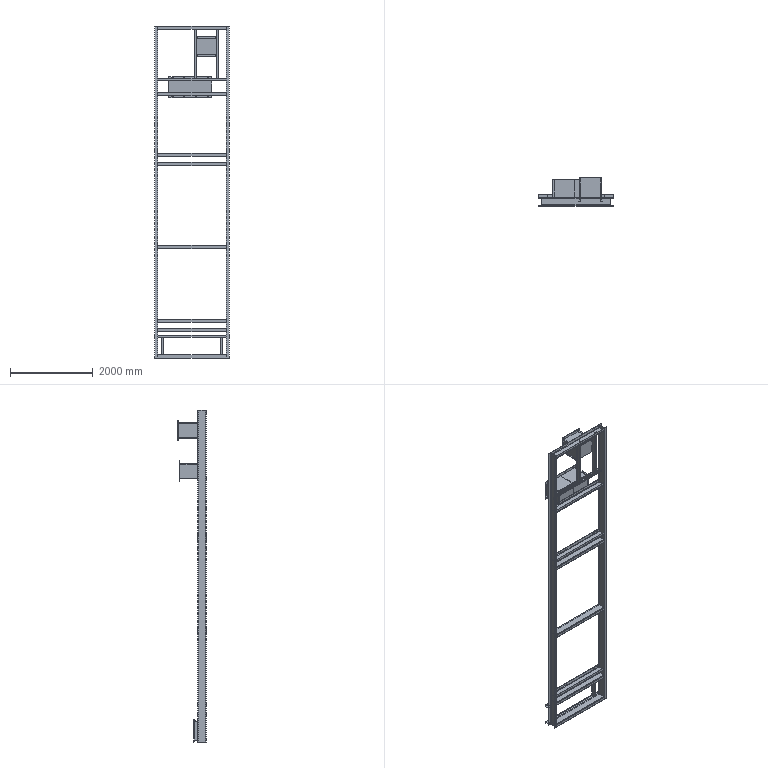Part | SolidWorks | features MoveFace 19, MoveCopyBody 18, ICE 10, MirrorSolid 9, WeldMemberFeat 7, 3DProfileFeature 3, Cut 3, DeleteBody 2, Shell 2, Punch 1, WeldmentFeature 1 | 26 solids | 436 faces | box 1791 x 685 x 8000 mm | volume 140497975 mm3 | plane 240 | cylinder 196 | commonest cylinder face diameters 24 x96 11 x20 22 x20 8.5 x18 17 x18 32 x16